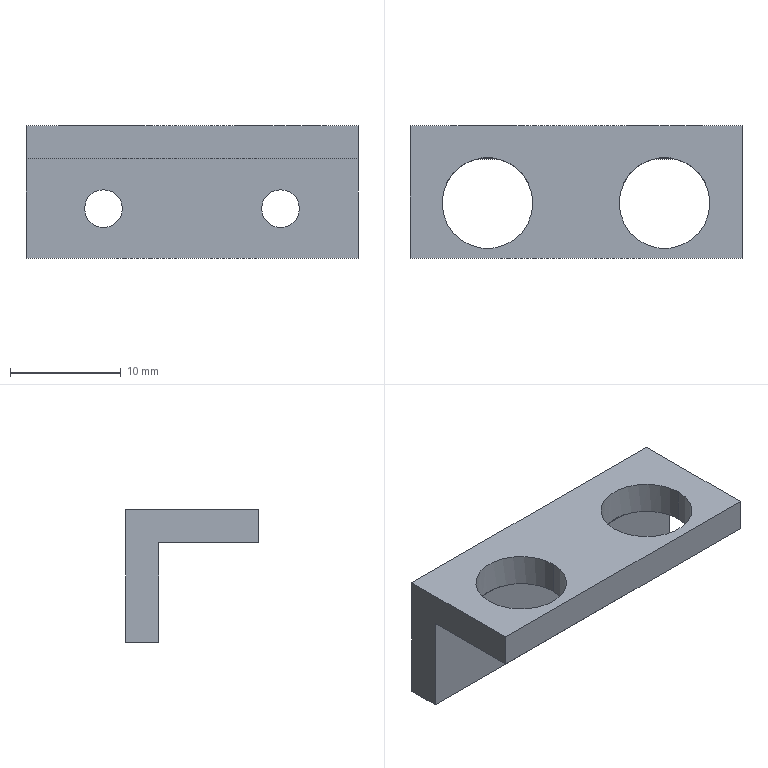NC program | NX | posted with a generic post | part box 30 x 12 x 12 mm
Lines 1848 to 1871 of 1871:
(PLANAR_MILL_COPY_1_COPY_COPY , TOOL : D6A45)
N3682 T01 M6
N3684 G54
N3686 G17 G0 G90 X0.766 Y-7.257 B0. C0. S7500 M3
N3688 G43 Z30. H1
N3690 Z1.
N3692 G94 G1 Z-1. F1250.
N3694 G3 X0. Y-6.9 R1.
N3696 G1 X-15.
N3698 G2 X-15.9 Y-6. R0.9
N3700 G1 Y6.
N3702 G2 X-15. Y6.9 R0.9
N3704 G1 X15.
N3706 G2 X15.9 Y6. R0.9
N3708 G1 Y-6.
N3710 G2 X15. Y-6.9 R0.9
N3712 G1 X0.
N3714 G3 X-0.766 Y-7.257 R1.
N3716 G1 Z1.
N3718 G0 Z30.
N3720 M5
N3722 M2